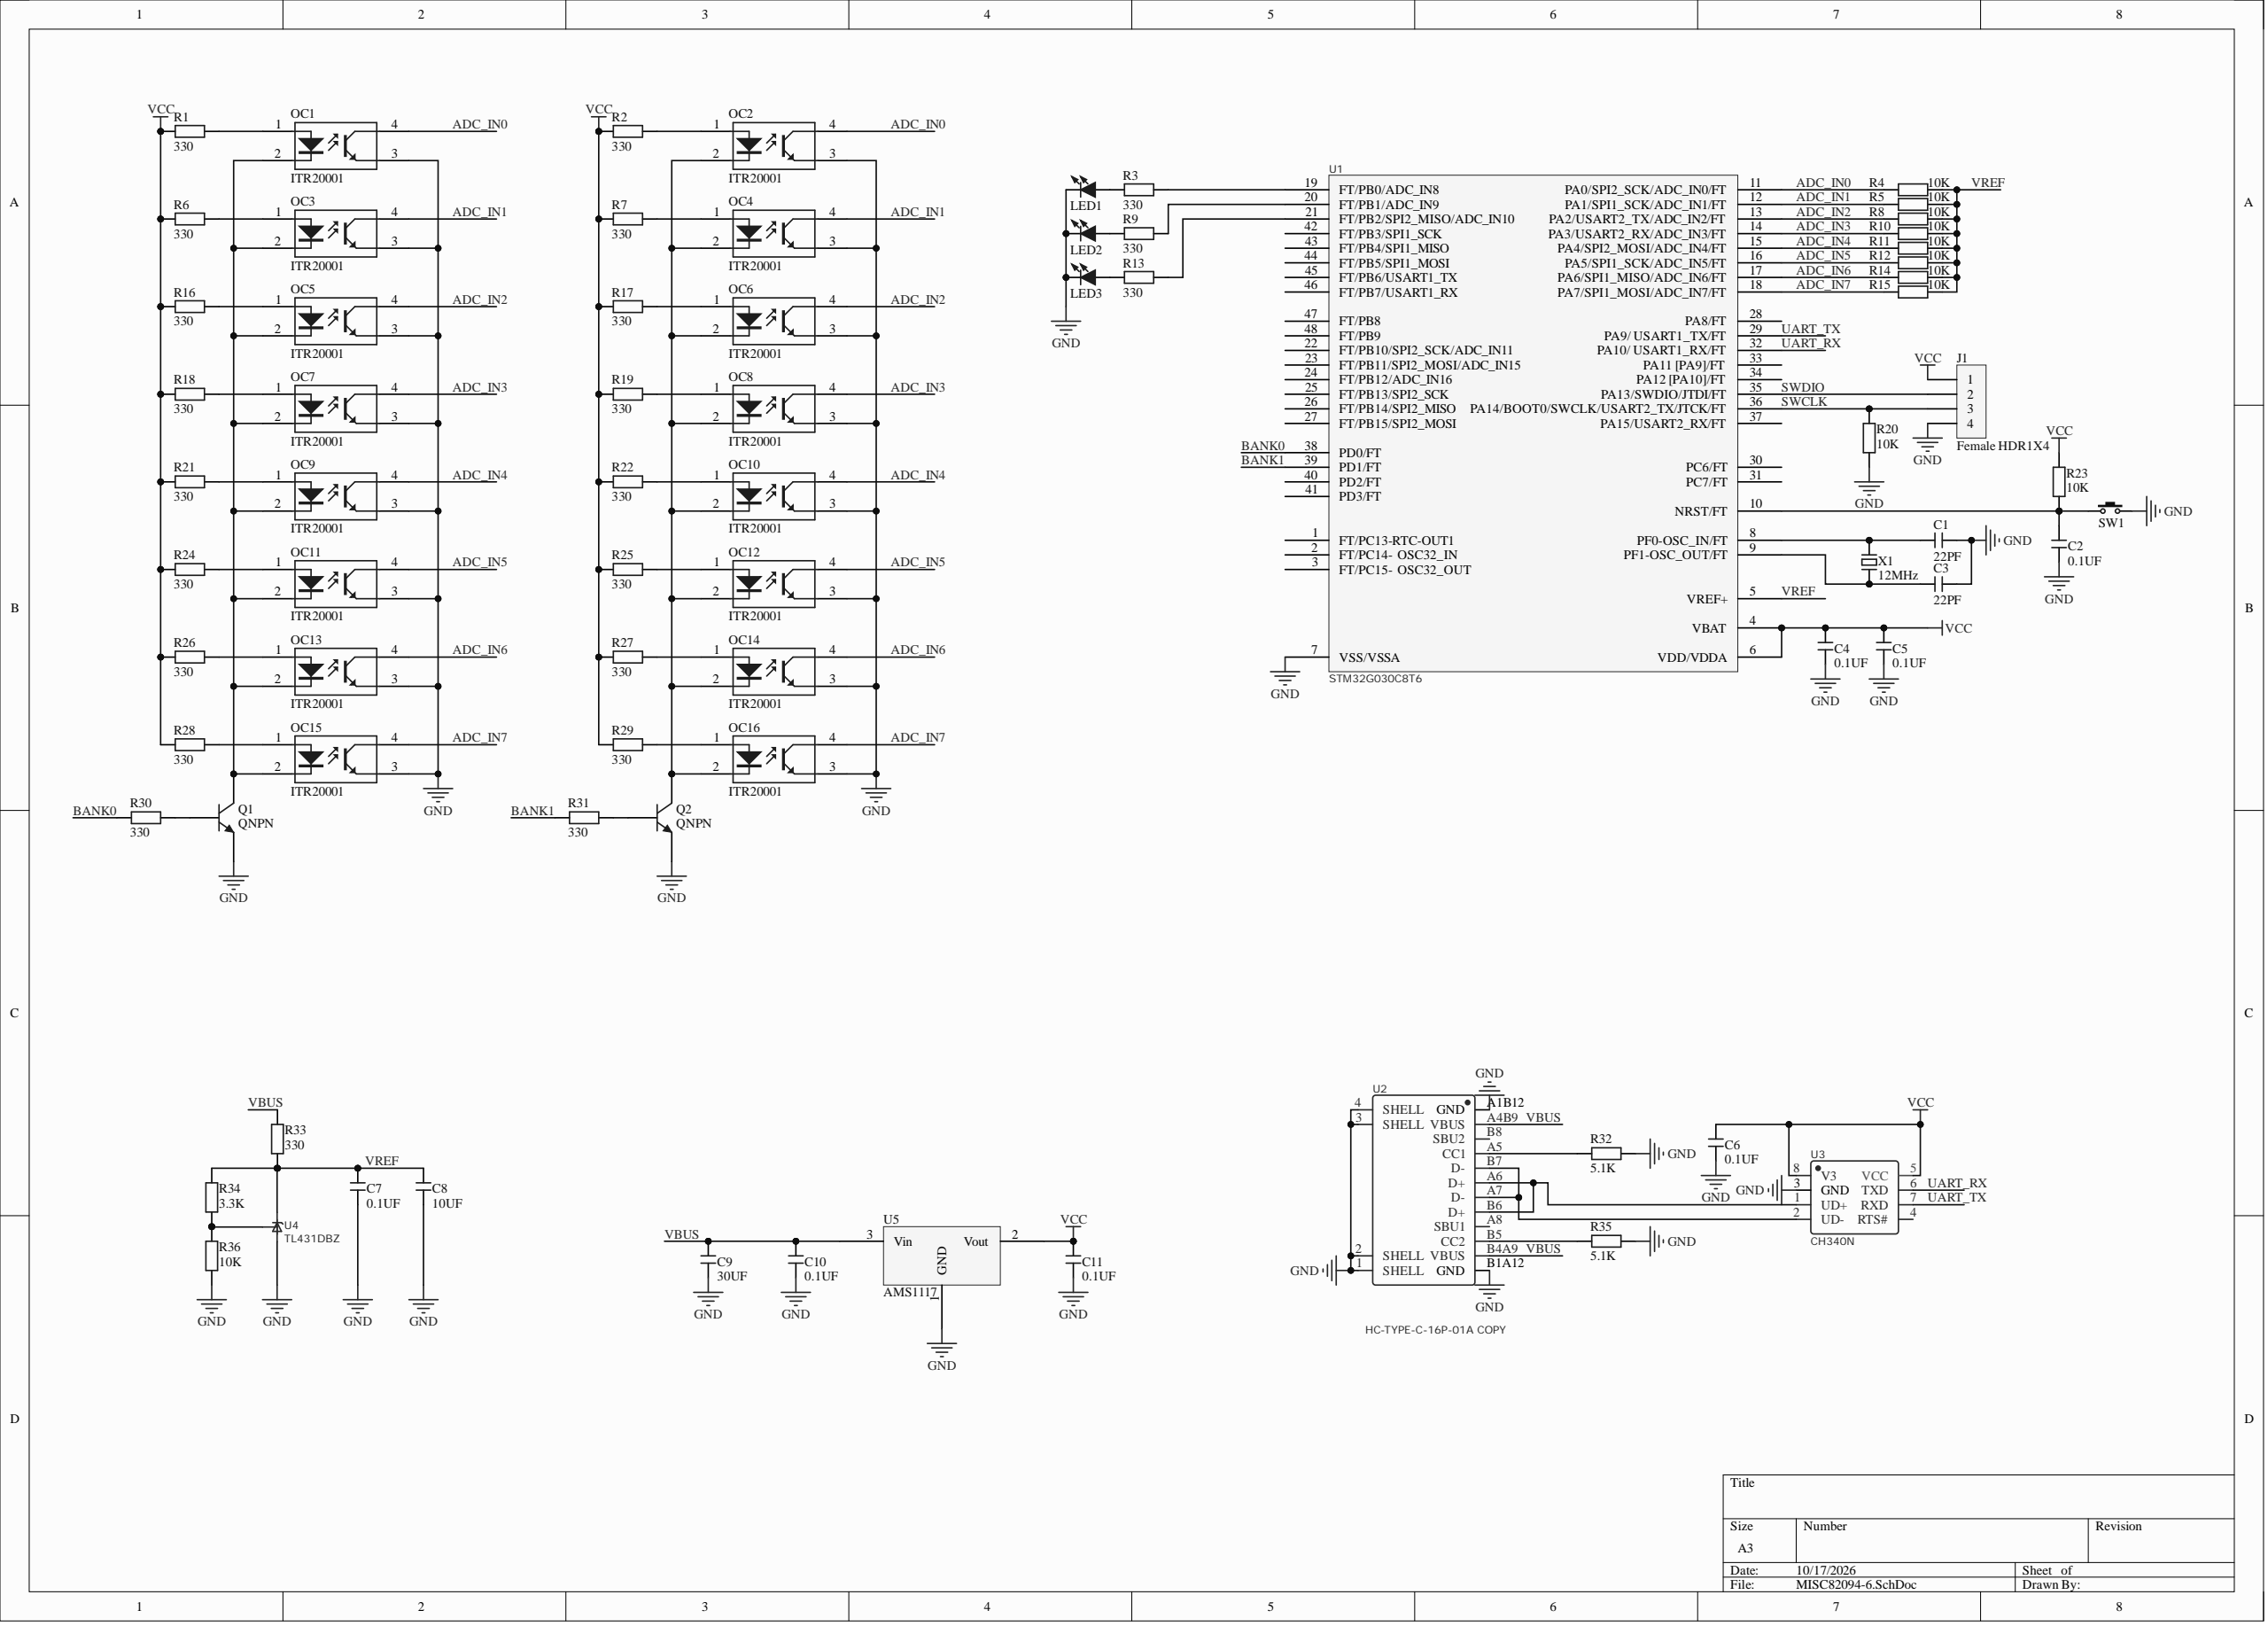Circuit board | Altium Designer | 76 parts | 52 nets
Bill of materials:
Comment,Description,Designator,Footprint,LibRef,Quantity
"22PF","SMD capacitor","C1, C3","C 0805_L","C","2"
"0.1UF","SMD capacitor","C2, C4, C5, C6, C7, C10, C11","C 0805_L","C","7"
"10UF","SMD capacitor","C8","C 1206_L","C","1"
"30UF","SMD capacitor","C9","C 1206_L","C","1"
"Female HDR1X4","","J1","Fe-HDR1X4/2.54-S","Female HDR1X4","1"
"Red","SMD LED","LED1, LED2, LED3","LED 0805G","LED-SMD","3"
"ITR20001","Linear optocoupler","OC1, OC2, OC3, OC4, OC5, OC6, OC7, OC8, OC9, OC10, OC11, OC12, OC13, OC14, OC15, OC16","SMD_PC817","PC817","16"
"QNPN","NPN Bipolar Transistor","Q1, Q2","SOT-23B_N","QNPN","2"
"330","SMD resistor","R1, R2, R3, R6, R7, R9, R13, R16, R17, R18, R19, R21, R22, R24, R25, R26, R27, R28, R29, R30, R31","R 0603_L","R","21"
"10K","SMD resistor","R4, R5, R8, R10, R11, R12, R14, R15, R20, R23, R36","R 0805_L","R","11"
"5.1K","SMD resistor","R32, R35","R 0805_L","R","2"
"330","SMD resistor","R33","R 0805_L","R","1"
"3.3K","SMD resistor","R34","R 0805_L","R","1"
"3x6x5","3x6 tact switch","SW1","TSW SMD-3*6*2.5","TSW 3x6","1"
"STM32G030C8T6","","U1","LQFP48_N","STM32G030C8T6","1"
"HC-TYPE-C-16P-01A COPY","","U2","USB-C-SMD_HC-TYPE-C-16P-01A","HC-TYPE-C-16P-01A COPY","1"
"CH340N","","U3","SOP8","CH340N","1"
"TL431DBZ","","U4","SOT-23","TL431DBZ","1"
"AMS1117","Three-terminal voltage regulator","U5","SOT223","AMS1117","1"
"12MHz","2-pin passive crystal oscillator","X1","OSC HC-49S","XTAL-2P","1"
Netlist (Protel format):
[
C1
C 0805_L
22PF



]
[
C2
C 0805_L
0.1UF



]
[
C3
C 0805_L
22PF



]
[
C4
C 0805_L
0.1UF



]
[
C5
C 0805_L
0.1UF



]
[
C6
C 0805_L
0.1UF



]
[
C7
C 0805_L
0.1UF



]
[
C8
C 1206_L
10UF



]
[
C9
C 1206_L
30UF



]
[
C10
C 0805_L
0.1UF



]
[
C11
C 0805_L
0.1UF



]
[
J1
Fe-HDR1X4/2.54-S
Female HDR1X4



]
[
LED1
LED 0805G
Red



]
[
LED2
LED 0805G
Red



]
[
LED3
LED 0805G
Red



]
[
OC1
SMD_PC817
ITR20001



]
[
OC2
SMD_PC817
ITR20001



]
[
OC3
SMD_PC817
ITR20001



]
[
OC4
SMD_PC817
ITR20001



]
[
OC5
SMD_PC817
ITR20001



]
[
OC6
SMD_PC817
ITR20001



]
[
OC7
SMD_PC817
ITR20001



]
[
OC8
SMD_PC817
ITR20001



]
[
OC9
SMD_PC817
ITR20001



]
[
OC10
SMD_PC817
ITR20001



]
[
OC11
SMD_PC817
ITR20001



]
[
OC12
SMD_PC817
ITR20001



]
[
OC13
SMD_PC817
ITR20001



]
[
OC14
SMD_PC817
ITR20001



]
[
OC15
SMD_PC817
ITR20001



]
[
OC16
SMD_PC817
ITR20001



]
[
Q1
SOT-23B_N
QNPN



]
[
Q2
SOT-23B_N
QNPN



]
[
R1
R 0603_L
330



]
[
R2
R 0603_L
330



]
[
R3
R 0603_L
330



]
[
R4
R 0805_L
10K



]
[
R5
R 0805_L
10K



]
[
R6
R 0603_L
330



]
[
R7
R 0603_L
330



]
[
R8
R 0805_L
10K



]
[
R9
R 0603_L
330



]
[
R10
R 0805_L
10K



]
[
R11
R 0805_L
10K



]
[
R12
R 0805_L
10K



]
[
R13
R 0603_L
330



]
[
R14
R 0805_L
10K



]
[
R15
R 0805_L
10K



]
[
R16
R 0603_L
330



]
[
R17
R 0603_L
330



]
[
R18
R 0603_L
330



]
[
R19
R 0603_L
330



]
[
R20
R 0805_L
10K



]
[
R21
R 0603_L
330



]
[
R22
R 0603_L
330



]
[
R23
R 0805_L
10K



]
[
R24
R 0603_L
330



]
[
R25
R 0603_L
330



]
[
R26
R 0603_L
330



]
[
R27
R 0603_L
330



]
[
R28
R 0603_L
330



]
[
R29
R 0603_L
330



]
[
R30
R 0603_L
330



]
[
R31
R 0603_L
330



]
[
R32
R 0805_L
5.1K



]
[
R33
R 0805_L
330



]
[
R34
R 0805_L
3.3K



]
[
R35
R 0805_L
5.1K



]
[
R36
R 0805_L
10K



]
[
SW1
TSW SMD-3*6*2.5
3x6x5



]
[
U1
LQFP48_N
STM32G030C8T6



]
[
U2
USB-C-SMD_HC-TYPE-C-16P-01A
HC-TYPE-C-16P-01A COPY



]
[
U3
SOP8
CH340N



]
[
U4
SOT-23
TL431DBZ



]
[
U5
SOT223
AMS1117



]
[
X1
OSC HC-49S
12MHz



]
(
VREF
C7-2
C8-2
R4-2
R5-2
R8-2
R10-2
R11-2
R12-2
R14-2
R15-2
R33-1
R34-2
U1-5
U4-2
)
(
VCC
C4-2
C5-2
C6-2
C11-2
J1-1
R1-1
R2-1
R6-1
R7-1
R16-1
R17-1
R18-1
R19-1
R21-1
R22-1
R23-2
R24-1
R25-1
R26-1
R27-1
R28-1
R29-1
U1-4
U1-6
U3-5
U3-8
U5-2
)
(
VBUS
C9-2
C10-2
R33-2
U2-A4B9
U2-B4A9
U5-3
)
(
UART_TX
U1-29
U3-7
)
(
UART_RX
U1-32
U3-6
)
(
SWDIO
J1-2
U1-35
)
(
SWCLK
J1-3
R20-2
U1-36
)
(
NetU2_A7
U2-A7
U2-B7
U3-2
)
(
NetU2_A6
U2-A6
U2-B6
U3-1
)
(
NetR35_2
R35-2
U2-B5
)
(
NetR34_1
R34-1
R36-2
U4-1
)
(
NetR32_2
R32-2
U2-A5
)
(
NetR13_2
R13-2
U1-21
)
(
NetR9_2
R9-2
U1-20
)
(
NetR3_2
R3-2
U1-19
)
(
NetQ2_2
Q2-2
R31-2
)
(
NetQ1_2
Q1-2
R30-2
)
(
NetOC16_1
OC16-1
R29-2
)
(
NetOC15_1
OC15-1
R28-2
)
(
NetOC14_1
OC14-1
R27-2
)
(
NetOC13_1
OC13-1
R26-2
)
(
NetOC12_1
OC12-1
R25-2
)
(
NetOC11_1
OC11-1
R24-2
)
(
NetOC10_1
OC10-1
R22-2
)
(
NetOC9_1
OC9-1
R21-2
)
(
NetOC8_1
OC8-1
R19-2
)
(
NetOC7_1
OC7-1
R18-2
)
(
NetOC6_1
OC6-1
R17-2
)
(
NetOC5_1
OC5-1
R16-2
)
(
NetOC4_1
OC4-1
R7-2
)
(
NetOC3_1
OC3-1
R6-2
)
(
NetOC2_2
OC2-2
OC4-2
OC6-2
OC8-2
OC10-2
OC12-2
OC14-2
OC16-2
Q2-1
)
(
NetOC2_1
OC2-1
R2-2
)
(
NetOC1_2
OC1-2
OC3-2
OC5-2
OC7-2
OC9-2
OC11-2
OC13-2
OC15-2
Q1-1
)
(
NetOC1_1
OC1-1
R1-2
)
(
NetLED3_1
LED3-1
R13-1
)
(
NetLED2_1
LED2-1
R9-1
)
(
NetLED1_1
LED1-1
R3-1
)
(
NetC3_1
C3-1
U1-9
X1-1
)
(
NetC2_2
C2-2
R23-1
SW1-1
U1-10
)
(
NetC1_2
C1-2
U1-8
X1-2
)
(
GND
C1-1
C2-1
C3-2
C4-1
C5-1
C6-1
C7-1
C8-1
C9-1
C10-1
C11-1
J1-4
LED1-2
LED2-2
LED3-2
OC1-3
OC2-3
OC3-3
OC4-3
OC5-3
OC6-3
OC7-3
OC8-3
OC9-3
OC10-3
OC11-3
OC12-3
OC13-3
OC14-3
OC15-3
OC16-3
Q1-3
Q2-3
R20-1
R32-1
R35-1
R36-1
SW1-2
U1-7
U2-1
U2-2
U2-3
U2-4
U2-A1B12
U2-B1A12
U3-3
U4-3
U5-1
)
(
BANK1
R31-1
U1-39
)
(
BANK0
R30-1
U1-38
)
(
ADC_IN7
OC15-4
OC16-4
R15-1
U1-18
)
(
ADC_IN6
OC13-4
OC14-4
R14-1
U1-17
)
(
ADC_IN5
OC11-4
OC12-4
R12-1
U1-16
)
(
ADC_IN4
OC9-4
OC10-4
R11-1
U1-15
)
(
ADC_IN3
OC7-4
OC8-4
R10-1
U1-14
)
(
ADC_IN2
OC5-4
OC6-4
R8-1
U1-13
)
(
ADC_IN1
OC3-4
OC4-4
R5-1
U1-12
)
(
ADC_IN0
OC1-4
OC2-4
R4-1
U1-11
)